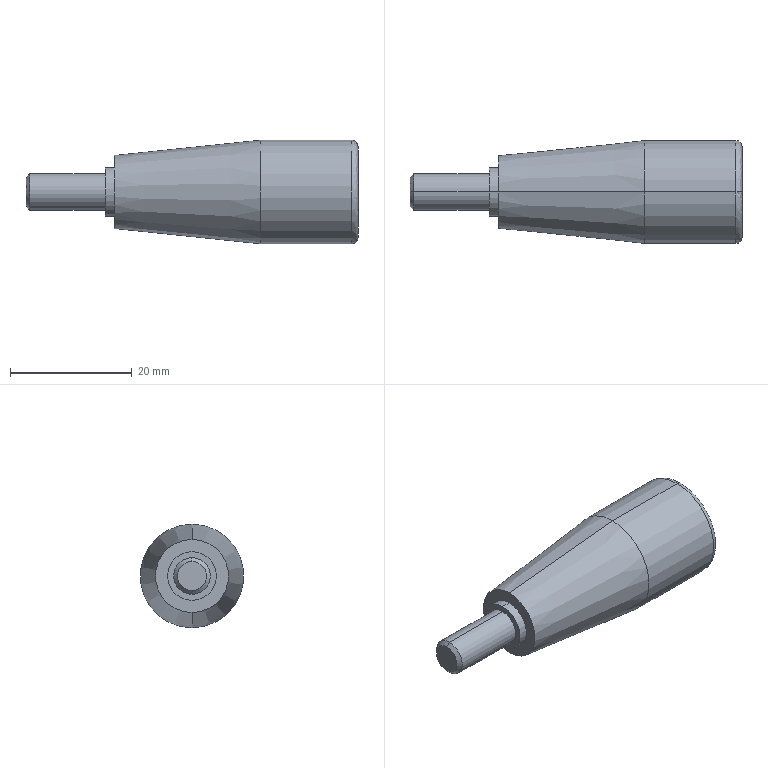Part | STEP file | GRAM6 | 1 solid | 20 faces | box 54.5 x 17 x 17 mm | volume 8003 mm3 | cylinder 8 | plane 6 | cone 4 | spline 2 | commonest cylinder face diameters 6 x2 6.5 x2 8 x2 17 x2
STEP:
#1=CARTESIAN_POINT('',(0.,0.,0.));
#2=DIRECTION('',(0.,0.,1.));
#3=DIRECTION('',(1.,0.,0.));
#4=AXIS2_PLACEMENT_3D('',#1,#2,#3);
#5=CARTESIAN_POINT('',(40.,0.,-7.5));
#6=VERTEX_POINT('',#5);
#7=CARTESIAN_POINT('',(40.,0.,7.5));
#8=VERTEX_POINT('',#7);
#9=CARTESIAN_POINT('',(40.,0.,-7.5));
#10=CARTESIAN_POINT('',(40.,-15.,-7.5));
#11=CARTESIAN_POINT('',(40.,-15.,7.5));
#12=CARTESIAN_POINT('',(40.,0.,7.5));
#13=(BOUNDED_CURVE()B_SPLINE_CURVE(3,(#9,#10,#11,#12),.UNSPECIFIED.,.F.,.F.)B_SPLINE_CURVE_WITH_KNOTS((4,4),(0.25,0.75),.PIECEWISE_BEZIER_KNOTS.)CURVE()GEOMETRIC_REPRESENTATION_ITEM()RATIONAL_B_SPLINE_CURVE((1.,0.3333,0.3333,1.))REPRESENTATION_ITEM(''));
#14=CARTESIAN_POINT('',(40.,0.,7.5));
#15=CARTESIAN_POINT('',(40.,-15.,7.5));
#16=CARTESIAN_POINT('',(40.,-15.,-7.5));
#17=CARTESIAN_POINT('',(40.,0.,-7.5));
#18=CARTESIAN_POINT('',(40.,0.,8.086));
#19=CARTESIAN_POINT('',(40.,-16.172,8.086));
#20=CARTESIAN_POINT('',(40.,-16.172,-8.086));
#21=CARTESIAN_POINT('',(40.,0.,-8.086));
#22=CARTESIAN_POINT('',(39.586,0.,8.5));
#23=CARTESIAN_POINT('',(39.586,-17.,8.5));
#24=CARTESIAN_POINT('',(39.586,-17.,-8.5));
#25=CARTESIAN_POINT('',(39.586,0.,-8.5));
#26=CARTESIAN_POINT('',(39.,0.,8.5));
#27=CARTESIAN_POINT('',(39.,-17.,8.5));
#28=CARTESIAN_POINT('',(39.,-17.,-8.5));
#29=CARTESIAN_POINT('',(39.,0.,-8.5));
#30=(BOUNDED_SURFACE()B_SPLINE_SURFACE(3,3,((#14,#15,#16,#17),(#18,#19,#20,#21),(#22,#23,#24,#25),(#26,#27,#28,#29)),.UNSPECIFIED.,.F.,.F.,.F.)B_SPLINE_SURFACE_WITH_KNOTS((4,4),(4,4),(0.,1.),(0.,1.),.PIECEWISE_BEZIER_KNOTS.)GEOMETRIC_REPRESENTATION_ITEM()RATIONAL_B_SPLINE_SURFACE(((1.,0.3333,0.3333,1.),(0.8047,0.2682,0.2682,0.8047),(0.8047,0.2682,0.2682,0.8047),(1.,0.3333,0.3333,1.)))REPRESENTATION_ITEM('')SURFACE());
#31=CARTESIAN_POINT('',(0.,1.));
#32=CARTESIAN_POINT('',(0.,0.));
#33=B_SPLINE_CURVE_WITH_KNOTS('',1,(#31,#32),.UNSPECIFIED.,.F.,.F.,(2,2),(0.25,0.75),.PIECEWISE_BEZIER_KNOTS.);
#34=(GEOMETRIC_REPRESENTATION_CONTEXT(2)PARAMETRIC_REPRESENTATION_CONTEXT()REPRESENTATION_CONTEXT('',''));
#35=DEFINITIONAL_REPRESENTATION('',(#33),#34);
#36=PCURVE('',#30,#35);
#37=CARTESIAN_POINT('',(40.,3.75,0.));
#38=DIRECTION('',(1.,0.,0.));
#39=DIRECTION('',(0.,0.,-1.));
#40=AXIS2_PLACEMENT_3D('',#37,#38,#39);
#41=PLANE('',#40);
#42=CARTESIAN_POINT('',(7.5,-3.75));
#43=CARTESIAN_POINT('',(7.5,-18.75));
#44=CARTESIAN_POINT('',(-7.5,-18.75));
#45=CARTESIAN_POINT('',(-7.5,-3.75));
#46=(BOUNDED_CURVE()B_SPLINE_CURVE(3,(#42,#43,#44,#45),.UNSPECIFIED.,.F.,.F.)B_SPLINE_CURVE_WITH_KNOTS((4,4),(0.25,0.75),.PIECEWISE_BEZIER_KNOTS.)CURVE()GEOMETRIC_REPRESENTATION_ITEM()RATIONAL_B_SPLINE_CURVE((1.,0.3333,0.3333,1.))REPRESENTATION_ITEM(''));
#47=(GEOMETRIC_REPRESENTATION_CONTEXT(2)PARAMETRIC_REPRESENTATION_CONTEXT()REPRESENTATION_CONTEXT('',''));
#48=DEFINITIONAL_REPRESENTATION('',(#46),#47);
#49=PCURVE('',#41,#48);
#50=SURFACE_CURVE('',#13,(#36,#49),.PCURVE_S1.);
#51=EDGE_CURVE('',#6,#8,#50,.T.);
#52=ORIENTED_EDGE('',*,*,#51,.T.);
#53=CARTESIAN_POINT('',(39.,0.,8.5));
#54=VERTEX_POINT('',#53);
#55=CARTESIAN_POINT('',(39.,0.,7.5));
#56=DIRECTION('',(0.,-1.,0.));
#57=DIRECTION('',(0.,0.,1.));
#58=AXIS2_PLACEMENT_3D('',#55,#56,#57);
#59=CIRCLE('',#58,1.);
#60=CARTESIAN_POINT('',(0.,0.));
#61=CARTESIAN_POINT('',(0.01683,0.));
#62=CARTESIAN_POINT('',(0.04999,0.));
#63=CARTESIAN_POINT('',(0.09843,0.));
#64=CARTESIAN_POINT('',(0.1457,0.));
#65=CARTESIAN_POINT('',(0.192,0.));
#66=CARTESIAN_POINT('',(0.2375,0.));
#67=CARTESIAN_POINT('',(0.2823,0.));
#68=CARTESIAN_POINT('',(0.3265,0.));
#69=CARTESIAN_POINT('',(0.3703,0.));
#70=CARTESIAN_POINT('',(0.4137,0.));
#71=CARTESIAN_POINT('',(0.4569,0.));
#72=CARTESIAN_POINT('',(0.5,0.));
#73=CARTESIAN_POINT('',(0.5431,0.));
#74=CARTESIAN_POINT('',(0.5863,0.));
#75=CARTESIAN_POINT('',(0.6297,0.));
#76=CARTESIAN_POINT('',(0.6735,0.));
#77=CARTESIAN_POINT('',(0.7177,0.));
#78=CARTESIAN_POINT('',(0.7625,0.));
#79=CARTESIAN_POINT('',(0.808,0.));
#80=CARTESIAN_POINT('',(0.8543,0.));
#81=CARTESIAN_POINT('',(0.9016,0.));
#82=CARTESIAN_POINT('',(0.95,0.));
#83=CARTESIAN_POINT('',(0.9832,0.));
#84=CARTESIAN_POINT('',(1.,0.));
#85=B_SPLINE_CURVE_WITH_KNOTS('',3,(#60,#61,#62,#63,#64,#65,#66,#67,#68,#69,#70,#71,#72,#73,#74,#75,#76,#77,#78,#79,#80,#81,#82,#83,#84),.UNSPECIFIED.,.F.,.F.,(4,1,1,1,1,1,1,1,1,1,1,1,1,1,1,1,1,1,1,1,1,1,4),(4.712,4.784,4.855,4.927,4.998,5.069,5.141,5.212,5.284,5.355,5.426,5.498,5.569,5.641,5.712,5.783,5.855,5.926,5.998,6.069,6.14,6.212,6.283),.QUASI_UNIFORM_KNOTS.);
#86=(GEOMETRIC_REPRESENTATION_CONTEXT(2)PARAMETRIC_REPRESENTATION_CONTEXT()REPRESENTATION_CONTEXT('',''));
#87=DEFINITIONAL_REPRESENTATION('',(#85),#86);
#88=PCURVE('',#30,#87);
#89=CARTESIAN_POINT('',(40.,0.,-7.5));
#90=CARTESIAN_POINT('',(40.,15.,-7.5));
#91=CARTESIAN_POINT('',(40.,15.,7.5));
#92=CARTESIAN_POINT('',(40.,0.,7.5));
#93=CARTESIAN_POINT('',(40.,0.,-8.086));
#94=CARTESIAN_POINT('',(40.,16.172,-8.086));
#95=CARTESIAN_POINT('',(40.,16.172,8.086));
#96=CARTESIAN_POINT('',(40.,0.,8.086));
#97=CARTESIAN_POINT('',(39.586,0.,-8.5));
#98=CARTESIAN_POINT('',(39.586,17.,-8.5));
#99=CARTESIAN_POINT('',(39.586,17.,8.5));
#100=CARTESIAN_POINT('',(39.586,0.,8.5));
#101=CARTESIAN_POINT('',(39.,0.,-8.5));
#102=CARTESIAN_POINT('',(39.,17.,-8.5));
#103=CARTESIAN_POINT('',(39.,17.,8.5));
#104=CARTESIAN_POINT('',(39.,0.,8.5));
#105=(BOUNDED_SURFACE()B_SPLINE_SURFACE(3,3,((#89,#90,#91,#92),(#93,#94,#95,#96),(#97,#98,#99,#100),(#101,#102,#103,#104)),.UNSPECIFIED.,.F.,.F.,.F.)B_SPLINE_SURFACE_WITH_KNOTS((4,4),(4,4),(0.,1.),(0.,1.),.PIECEWISE_BEZIER_KNOTS.)GEOMETRIC_REPRESENTATION_ITEM()RATIONAL_B_SPLINE_SURFACE(((1.,0.3333,0.3333,1.),(0.8047,0.2682,0.2682,0.8047),(0.8047,0.2682,0.2682,0.8047),(1.,0.3333,0.3333,1.)))REPRESENTATION_ITEM('')SURFACE());
#106=CARTESIAN_POINT('',(0.,1.));
#107=CARTESIAN_POINT('',(0.01683,1.));
#108=CARTESIAN_POINT('',(0.04999,1.));
#109=CARTESIAN_POINT('',(0.09843,1.));
#110=CARTESIAN_POINT('',(0.1457,1.));
#111=CARTESIAN_POINT('',(0.192,1.));
#112=CARTESIAN_POINT('',(0.2375,1.));
#113=CARTESIAN_POINT('',(0.2823,1.));
#114=CARTESIAN_POINT('',(0.3265,1.));
#115=CARTESIAN_POINT('',(0.3703,1.));
#116=CARTESIAN_POINT('',(0.4137,1.));
#117=CARTESIAN_POINT('',(0.4569,1.));
#118=CARTESIAN_POINT('',(0.5,1.));
#119=CARTESIAN_POINT('',(0.5431,1.));
#120=CARTESIAN_POINT('',(0.5863,1.));
#121=CARTESIAN_POINT('',(0.6297,1.));
#122=CARTESIAN_POINT('',(0.6735,1.));
#123=CARTESIAN_POINT('',(0.7177,1.));
#124=CARTESIAN_POINT('',(0.7625,1.));
#125=CARTESIAN_POINT('',(0.808,1.));
#126=CARTESIAN_POINT('',(0.8543,1.));
#127=CARTESIAN_POINT('',(0.9016,1.));
#128=CARTESIAN_POINT('',(0.95,1.));
#129=CARTESIAN_POINT('',(0.9832,1.));
#130=CARTESIAN_POINT('',(1.,1.));
#131=B_SPLINE_CURVE_WITH_KNOTS('',3,(#106,#107,#108,#109,#110,#111,#112,#113,#114,#115,#116,#117,#118,#119,#120,#121,#122,#123,#124,#125,#126,#127,#128,#129,#130),.UNSPECIFIED.,.F.,.F.,(4,1,1,1,1,1,1,1,1,1,1,1,1,1,1,1,1,1,1,1,1,1,4),(4.712,4.784,4.855,4.927,4.998,5.069,5.141,5.212,5.284,5.355,5.426,5.498,5.569,5.641,5.712,5.783,5.855,5.926,5.998,6.069,6.14,6.212,6.283),.QUASI_UNIFORM_KNOTS.);
#132=(GEOMETRIC_REPRESENTATION_CONTEXT(2)PARAMETRIC_REPRESENTATION_CONTEXT()REPRESENTATION_CONTEXT('',''));
#133=DEFINITIONAL_REPRESENTATION('',(#131),#132);
#134=PCURVE('',#105,#133);
#135=SURFACE_CURVE('',#59,(#88,#134),.PCURVE_S1.);
#136=EDGE_CURVE('',#8,#54,#135,.T.);
#137=ORIENTED_EDGE('',*,*,#136,.T.);
#138=CARTESIAN_POINT('',(39.,0.,-8.5));
#139=VERTEX_POINT('',#138);
#140=CARTESIAN_POINT('',(39.,0.,0.));
#141=DIRECTION('',(-1.,0.,0.));
#142=DIRECTION('',(0.,0.,-1.));
#143=AXIS2_PLACEMENT_3D('',#140,#141,#142);
#144=CIRCLE('',#143,8.5);
#145=CARTESIAN_POINT('',(1.,1.));
#146=CARTESIAN_POINT('',(1.,0.9763));
#147=CARTESIAN_POINT('',(1.,0.9319));
#148=CARTESIAN_POINT('',(1.,0.8733));
#149=CARTESIAN_POINT('',(1.,0.8206));
#150=CARTESIAN_POINT('',(1.,0.7724));
#151=CARTESIAN_POINT('',(1.,0.7279));
#152=CARTESIAN_POINT('',(1.,0.6861));
#153=CARTESIAN_POINT('',(1.,0.6465));
#154=CARTESIAN_POINT('',(1.,0.6086));
#155=CARTESIAN_POINT('',(1.,0.5718));
#156=CARTESIAN_POINT('',(1.,0.5357));
#157=CARTESIAN_POINT('',(1.,0.5));
#158=CARTESIAN_POINT('',(1.,0.4643));
#159=CARTESIAN_POINT('',(1.,0.4282));
#160=CARTESIAN_POINT('',(1.,0.3914));
#161=CARTESIAN_POINT('',(1.,0.3535));
#162=CARTESIAN_POINT('',(1.,0.3139));
#163=CARTESIAN_POINT('',(1.,0.2721));
#164=CARTESIAN_POINT('',(1.,0.2276));
#165=CARTESIAN_POINT('',(1.,0.1794));
#166=CARTESIAN_POINT('',(1.,0.1267));
#167=CARTESIAN_POINT('',(1.,0.06805));
#168=CARTESIAN_POINT('',(1.,0.02375));
#169=CARTESIAN_POINT('',(1.,0.));
#170=B_SPLINE_CURVE_WITH_KNOTS('',3,(#145,#146,#147,#148,#149,#150,#151,#152,#153,#154,#155,#156,#157,#158,#159,#160,#161,#162,#163,#164,#165,#166,#167,#168,#169),.UNSPECIFIED.,.F.,.F.,(4,1,1,1,1,1,1,1,1,1,1,1,1,1,1,1,1,1,1,1,1,1,4),(0.,0.1428,0.2856,0.4284,0.5712,0.714,0.8568,0.9996,1.142,1.285,1.428,1.571,1.714,1.856,1.999,2.142,2.285,2.428,2.57,2.713,2.856,2.999,3.142),.QUASI_UNIFORM_KNOTS.);
#171=(GEOMETRIC_REPRESENTATION_CONTEXT(2)PARAMETRIC_REPRESENTATION_CONTEXT()REPRESENTATION_CONTEXT('',''));
#172=DEFINITIONAL_REPRESENTATION('',(#170),#171);
#173=PCURVE('',#30,#172);
#174=CARTESIAN_POINT('',(31.5,0.,0.));
#175=DIRECTION('',(1.,0.,0.));
#176=DIRECTION('',(0.,0.,-1.));
#177=AXIS2_PLACEMENT_3D('',#174,#175,#176);
#178=CYLINDRICAL_SURFACE('',#177,8.5);
#179=CARTESIAN_POINT('',(6.283,7.5));
#180=DIRECTION('',(-1.,0.));
#181=VECTOR('',#180,1.);
#182=LINE('',#179,#181);
#183=(GEOMETRIC_REPRESENTATION_CONTEXT(2)PARAMETRIC_REPRESENTATION_CONTEXT()REPRESENTATION_CONTEXT('',''));
#184=DEFINITIONAL_REPRESENTATION('',(#182),#183);
#185=PCURVE('',#178,#184);
#186=SURFACE_CURVE('',#144,(#173,#185),.PCURVE_S1.);
#187=EDGE_CURVE('',#139,#54,#186,.T.);
#188=ORIENTED_EDGE('',*,*,#187,.F.);
#189=CARTESIAN_POINT('',(39.,0.,-7.5));
#190=DIRECTION('',(0.,1.,0.));
#191=DIRECTION('',(0.,0.,-1.));
#192=AXIS2_PLACEMENT_3D('',#189,#190,#191);
#193=CIRCLE('',#192,1.);
#194=CARTESIAN_POINT('',(0.,1.));
#195=CARTESIAN_POINT('',(0.01683,1.));
#196=CARTESIAN_POINT('',(0.04999,1.));
#197=CARTESIAN_POINT('',(0.09843,1.));
#198=CARTESIAN_POINT('',(0.1457,1.));
#199=CARTESIAN_POINT('',(0.192,1.));
#200=CARTESIAN_POINT('',(0.2375,1.));
#201=CARTESIAN_POINT('',(0.2823,1.));
#202=CARTESIAN_POINT('',(0.3265,1.));
#203=CARTESIAN_POINT('',(0.3703,1.));
#204=CARTESIAN_POINT('',(0.4137,1.));
#205=CARTESIAN_POINT('',(0.4569,1.));
#206=CARTESIAN_POINT('',(0.5,1.));
#207=CARTESIAN_POINT('',(0.5431,1.));
#208=CARTESIAN_POINT('',(0.5863,1.));
#209=CARTESIAN_POINT('',(0.6297,1.));
#210=CARTESIAN_POINT('',(0.6735,1.));
#211=CARTESIAN_POINT('',(0.7177,1.));
#212=CARTESIAN_POINT('',(0.7625,1.));
#213=CARTESIAN_POINT('',(0.808,1.));
#214=CARTESIAN_POINT('',(0.8543,1.));
#215=CARTESIAN_POINT('',(0.9016,1.));
#216=CARTESIAN_POINT('',(0.95,1.));
#217=CARTESIAN_POINT('',(0.9832,1.));
#218=CARTESIAN_POINT('',(1.,1.));
#219=B_SPLINE_CURVE_WITH_KNOTS('',3,(#194,#195,#196,#197,#198,#199,#200,#201,#202,#203,#204,#205,#206,#207,#208,#209,#210,#211,#212,#213,#214,#215,#216,#217,#218),.UNSPECIFIED.,.F.,.F.,(4,1,1,1,1,1,1,1,1,1,1,1,1,1,1,1,1,1,1,1,1,1,4),(4.712,4.784,4.855,4.927,4.998,5.069,5.141,5.212,5.284,5.355,5.426,5.498,5.569,5.641,5.712,5.783,5.855,5.926,5.998,6.069,6.14,6.212,6.283),.QUASI_UNIFORM_KNOTS.);
#220=(GEOMETRIC_REPRESENTATION_CONTEXT(2)PARAMETRIC_REPRESENTATION_CONTEXT()REPRESENTATION_CONTEXT('',''));
#221=DEFINITIONAL_REPRESENTATION('',(#219),#220);
#222=PCURVE('',#30,#221);
#223=CARTESIAN_POINT('',(0.,0.));
#224=CARTESIAN_POINT('',(0.01683,0.));
#225=CARTESIAN_POINT('',(0.04999,0.));
#226=CARTESIAN_POINT('',(0.09843,0.));
#227=CARTESIAN_POINT('',(0.1457,0.));
#228=CARTESIAN_POINT('',(0.192,0.));
#229=CARTESIAN_POINT('',(0.2375,0.));
#230=CARTESIAN_POINT('',(0.2823,0.));
#231=CARTESIAN_POINT('',(0.3265,0.));
#232=CARTESIAN_POINT('',(0.3703,0.));
#233=CARTESIAN_POINT('',(0.4137,0.));
#234=CARTESIAN_POINT('',(0.4569,0.));
#235=CARTESIAN_POINT('',(0.5,0.));
#236=CARTESIAN_POINT('',(0.5431,0.));
#237=CARTESIAN_POINT('',(0.5863,0.));
#238=CARTESIAN_POINT('',(0.6297,0.));
#239=CARTESIAN_POINT('',(0.6735,0.));
#240=CARTESIAN_POINT('',(0.7177,0.));
#241=CARTESIAN_POINT('',(0.7625,0.));
#242=CARTESIAN_POINT('',(0.808,0.));
#243=CARTESIAN_POINT('',(0.8543,0.));
#244=CARTESIAN_POINT('',(0.9016,0.));
#245=CARTESIAN_POINT('',(0.95,0.));
#246=CARTESIAN_POINT('',(0.9832,0.));
#247=CARTESIAN_POINT('',(1.,0.));
#248=B_SPLINE_CURVE_WITH_KNOTS('',3,(#223,#224,#225,#226,#227,#228,#229,#230,#231,#232,#233,#234,#235,#236,#237,#238,#239,#240,#241,#242,#243,#244,#245,#246,#247),.UNSPECIFIED.,.F.,.F.,(4,1,1,1,1,1,1,1,1,1,1,1,1,1,1,1,1,1,1,1,1,1,4),(4.712,4.784,4.855,4.927,4.998,5.069,5.141,5.212,5.284,5.355,5.426,5.498,5.569,5.641,5.712,5.783,5.855,5.926,5.998,6.069,6.14,6.212,6.283),.QUASI_UNIFORM_KNOTS.);
#249=(GEOMETRIC_REPRESENTATION_CONTEXT(2)PARAMETRIC_REPRESENTATION_CONTEXT()REPRESENTATION_CONTEXT('',''));
#250=DEFINITIONAL_REPRESENTATION('',(#248),#249);
#251=PCURVE('',#105,#250);
#252=SURFACE_CURVE('',#193,(#222,#251),.PCURVE_S1.);
#253=EDGE_CURVE('',#6,#139,#252,.T.);
#254=ORIENTED_EDGE('',*,*,#253,.F.);
#255=EDGE_LOOP('',(#52,#137,#188,#254));
#256=FACE_BOUND('',#255,.T.);
#257=ADVANCED_FACE('',(#256),#30,.T.);
#258=CARTESIAN_POINT('',(0.,0.,-6.));
#259=VERTEX_POINT('',#258);
#260=CARTESIAN_POINT('',(0.,0.,6.));
#261=VERTEX_POINT('',#260);
#262=CARTESIAN_POINT('',(0.,0.,0.));
#263=DIRECTION('',(1.,0.,0.));
#264=DIRECTION('',(0.,0.,-1.));
#265=AXIS2_PLACEMENT_3D('',#262,#263,#264);
#266=CIRCLE('',#265,6.);
#267=CARTESIAN_POINT('',(24.,0.,0.));
#268=DIRECTION('',(1.,0.,0.));
#269=DIRECTION('',(0.,0.,-1.));
#270=AXIS2_PLACEMENT_3D('',#267,#268,#269);
#271=CONICAL_SURFACE('',#270,8.5,0.1038);
#272=CARTESIAN_POINT('',(0.,-24.));
#273=DIRECTION('',(1.,0.));
#274=VECTOR('',#273,1.);
#275=LINE('',#272,#274);
#276=(GEOMETRIC_REPRESENTATION_CONTEXT(2)PARAMETRIC_REPRESENTATION_CONTEXT()REPRESENTATION_CONTEXT('',''));
#277=DEFINITIONAL_REPRESENTATION('',(#275),#276);
#278=PCURVE('',#271,#277);
#279=CARTESIAN_POINT('',(0.,3.,0.));
#280=DIRECTION('',(-1.,0.,0.));
#281=DIRECTION('',(0.,0.,1.));
#282=AXIS2_PLACEMENT_3D('',#279,#280,#281);
#283=PLANE('',#282);
#284=CARTESIAN_POINT('',(-6.,-3.));
#285=CARTESIAN_POINT('',(-6.,7.392));
#286=CARTESIAN_POINT('',(3.,2.196));
#287=CARTESIAN_POINT('',(12.,-3.));
#288=CARTESIAN_POINT('',(3.,-8.196));
#289=CARTESIAN_POINT('',(-6.,-13.392));
#290=CARTESIAN_POINT('',(-6.,-3.));
#291=(BOUNDED_CURVE()B_SPLINE_CURVE(2,(#284,#285,#286,#287,#288,#289,#290),.UNSPECIFIED.,.T.,.F.)B_SPLINE_CURVE_WITH_KNOTS((1,2,2,2,2,1),(-2.094,0.,2.094,4.189,6.283,8.378),.UNSPECIFIED.)CURVE()GEOMETRIC_REPRESENTATION_ITEM()RATIONAL_B_SPLINE_CURVE((1.,0.5,1.,0.5,1.,0.5,1.))REPRESENTATION_ITEM(''));
#292=(GEOMETRIC_REPRESENTATION_CONTEXT(2)PARAMETRIC_REPRESENTATION_CONTEXT()REPRESENTATION_CONTEXT('',''));
#293=DEFINITIONAL_REPRESENTATION('',(#291),#292);
#294=PCURVE('',#283,#293);
#295=SURFACE_CURVE('',#266,(#278,#294),.PCURVE_S1.);
#296=EDGE_CURVE('',#259,#261,#295,.T.);
#297=ORIENTED_EDGE('',*,*,#296,.T.);
#298=CARTESIAN_POINT('',(24.,0.,8.5));
#299=VERTEX_POINT('',#298);
#300=CARTESIAN_POINT('',(24.,0.,8.5));
#301=DIRECTION('',(0.9946,0.,0.1036));
#302=VECTOR('',#301,1.);
#303=LINE('',#300,#302);
#304=CARTESIAN_POINT('',(3.142,0.));
#305=DIRECTION('',(0.,1.));
#306=VECTOR('',#305,1.);
#307=LINE('',#304,#306);
#308=(GEOMETRIC_REPRESENTATION_CONTEXT(2)PARAMETRIC_REPRESENTATION_CONTEXT()REPRESENTATION_CONTEXT('',''));
#309=DEFINITIONAL_REPRESENTATION('',(#307),#308);
#310=PCURVE('',#271,#309);
#311=CARTESIAN_POINT('',(24.,0.,0.));
#312=DIRECTION('',(1.,0.,0.));
#313=DIRECTION('',(0.,0.,-1.));
#314=AXIS2_PLACEMENT_3D('',#311,#312,#313);
#315=CONICAL_SURFACE('',#314,8.5,0.1038);
#316=CARTESIAN_POINT('',(3.142,0.));
#317=DIRECTION('',(0.,1.));
#318=VECTOR('',#317,1.);
#319=LINE('',#316,#318);
#320=(GEOMETRIC_REPRESENTATION_CONTEXT(2)PARAMETRIC_REPRESENTATION_CONTEXT()REPRESENTATION_CONTEXT('',''));
#321=DEFINITIONAL_REPRESENTATION('',(#319),#320);
#322=PCURVE('',#315,#321);
#323=SURFACE_CURVE('',#303,(#310,#322),.PCURVE_S1.);
#324=EDGE_CURVE('',#261,#299,#323,.T.);
#325=ORIENTED_EDGE('',*,*,#324,.T.);
#326=CARTESIAN_POINT('',(24.,0.,-8.5));
#327=VERTEX_POINT('',#326);
#328=CARTESIAN_POINT('',(24.,0.,0.));
#329=DIRECTION('',(-1.,0.,0.));
#330=DIRECTION('',(0.,1.,0.));
#331=AXIS2_PLACEMENT_3D('',#328,#329,#330);
#332=CIRCLE('',#331,8.5);
#333=CARTESIAN_POINT('',(7.854,0.));
#334=DIRECTION('',(-1.,0.));
#335=VECTOR('',#334,1.);
#336=LINE('',#333,#335);
#337=(GEOMETRIC_REPRESENTATION_CONTEXT(2)PARAMETRIC_REPRESENTATION_CONTEXT()REPRESENTATION_CONTEXT('',''));
#338=DEFINITIONAL_REPRESENTATION('',(#336),#337);
#339=PCURVE('',#271,#338);
#340=CARTESIAN_POINT('',(31.5,0.,0.));
#341=DIRECTION('',(1.,0.,0.));
#342=DIRECTION('',(0.,0.,-1.));
#343=AXIS2_PLACEMENT_3D('',#340,#341,#342);
#344=CYLINDRICAL_SURFACE('',#343,8.5);
#345=CARTESIAN_POINT('',(7.854,-7.5));
#346=DIRECTION('',(-1.,0.));
#347=VECTOR('',#346,1.);
#348=LINE('',#345,#347);
#349=(GEOMETRIC_REPRESENTATION_CONTEXT(2)PARAMETRIC_REPRESENTATION_CONTEXT()REPRESENTATION_CONTEXT('',''));
#350=DEFINITIONAL_REPRESENTATION('',(#348),#349);
#351=PCURVE('',#344,#350);
#352=SURFACE_CURVE('',#332,(#339,#351),.PCURVE_S1.);
#353=EDGE_CURVE('',#299,#327,#352,.T.);
#354=ORIENTED_EDGE('',*,*,#353,.T.);
#355=CARTESIAN_POINT('',(24.,0.,-8.5));
#356=DIRECTION('',(0.9946,0.,-0.1036));
#357=VECTOR('',#356,1.);
#358=LINE('',#355,#357);
#359=CARTESIAN_POINT('',(0.,0.));
#360=DIRECTION('',(0.,1.));
#361=VECTOR('',#360,1.);
#362=LINE('',#359,#361);
#363=(GEOMETRIC_REPRESENTATION_CONTEXT(2)PARAMETRIC_REPRESENTATION_CONTEXT()REPRESENTATION_CONTEXT('',''));
#364=DEFINITIONAL_REPRESENTATION('',(#362),#363);
#365=PCURVE('',#271,#364);
#366=CARTESIAN_POINT('',(6.283,0.));
#367=DIRECTION('',(0.,1.));
#368=VECTOR('',#367,1.);
#369=LINE('',#366,#368);
#370=(GEOMETRIC_REPRESENTATION_CONTEXT(2)PARAMETRIC_REPRESENTATION_CONTEXT()REPRESENTATION_CONTEXT('',''));
#371=DEFINITIONAL_REPRESENTATION('',(#369),#370);
#372=PCURVE('',#315,#371);
#373=SURFACE_CURVE('',#358,(#365,#372),.PCURVE_S1.);
#374=EDGE_CURVE('',#259,#327,#373,.T.);
#375=ORIENTED_EDGE('',*,*,#374,.F.);
#376=EDGE_LOOP('',(#297,#325,#354,#375));
#377=FACE_BOUND('',#376,.T.);
#378=ADVANCED_FACE('',(#377),#271,.T.);
#379=ORIENTED_EDGE('',*,*,#353,.F.);
#380=CARTESIAN_POINT('',(31.5,0.,8.5));
#381=DIRECTION('',(1.,0.,0.));
#382=VECTOR('',#381,1.);
#383=LINE('',#380,#382);
#384=CARTESIAN_POINT('',(3.142,0.));
#385=DIRECTION('',(0.,1.));
#386=VECTOR('',#385,1.);
#387=LINE('',#384,#386);
#388=(GEOMETRIC_REPRESENTATION_CONTEXT(2)PARAMETRIC_REPRESENTATION_CONTEXT()REPRESENTATION_CONTEXT('',''));
#389=DEFINITIONAL_REPRESENTATION('',(#387),#388);
#390=PCURVE('',#344,#389);
#391=CARTESIAN_POINT('',(3.142,0.));
#392=DIRECTION('',(0.,1.));
#393=VECTOR('',#392,1.);
#394=LINE('',#391,#393);
#395=(GEOMETRIC_REPRESENTATION_CONTEXT(2)PARAMETRIC_REPRESENTATION_CONTEXT()REPRESENTATION_CONTEXT('',''));
#396=DEFINITIONAL_REPRESENTATION('',(#394),#395);
#397=PCURVE('',#178,#396);
#398=SURFACE_CURVE('',#383,(#390,#397),.PCURVE_S1.);
#399=EDGE_CURVE('',#299,#54,#398,.T.);
#400=ORIENTED_EDGE('',*,*,#399,.T.);
#401=CARTESIAN_POINT('',(39.,0.,0.));
#402=DIRECTION('',(-1.,0.,0.));
#403=DIRECTION('',(0.,0.,-1.));
#404=AXIS2_PLACEMENT_3D('',#401,#402,#403);
#405=CIRCLE('',#404,8.5);
#406=CARTESIAN_POINT('',(6.283,7.5));
#407=DIRECTION('',(-1.,0.));
#408=VECTOR('',#407,1.);
#409=LINE('',#406,#408);
#410=(GEOMETRIC_REPRESENTATION_CONTEXT(2)PARAMETRIC_REPRESENTATION_CONTEXT()REPRESENTATION_CONTEXT('',''));
#411=DEFINITIONAL_REPRESENTATION('',(#409),#410);
#412=PCURVE('',#344,#411);
#413=CARTESIAN_POINT('',(1.,1.));
#414=CARTESIAN_POINT('',(1.,0.9763));
#415=CARTESIAN_POINT('',(1.,0.9319));
#416=CARTESIAN_POINT('',(1.,0.8733));
#417=CARTESIAN_POINT('',(1.,0.8206));
#418=CARTESIAN_POINT('',(1.,0.7724));
#419=CARTESIAN_POINT('',(1.,0.7279));
#420=CARTESIAN_POINT('',(1.,0.6861));
#421=CARTESIAN_POINT('',(1.,0.6465));
#422=CARTESIAN_POINT('',(1.,0.6086));
#423=CARTESIAN_POINT('',(1.,0.5718));
#424=CARTESIAN_POINT('',(1.,0.5357));
#425=CARTESIAN_POINT('',(1.,0.5));
#426=CARTESIAN_POINT('',(1.,0.4643));
#427=CARTESIAN_POINT('',(1.,0.4282));
#428=CARTESIAN_POINT('',(1.,0.3914));
#429=CARTESIAN_POINT('',(1.,0.3535));
#430=CARTESIAN_POINT('',(1.,0.3139));
#431=CARTESIAN_POINT('',(1.,0.2721));
#432=CARTESIAN_POINT('',(1.,0.2276));
#433=CARTESIAN_POINT('',(1.,0.1794));
#434=CARTESIAN_POINT('',(1.,0.1267));
#435=CARTESIAN_POINT('',(1.,0.06805));
#436=CARTESIAN_POINT('',(1.,0.02375));
#437=CARTESIAN_POINT('',(1.,0.));
#438=B_SPLINE_CURVE_WITH_KNOTS('',3,(#413,#414,#415,#416,#417,#418,#419,#420,#421,#422,#423,#424,#425,#426,#427,#428,#429,#430,#431,#432,#433,#434,#435,#436,#437),.UNSPECIFIED.,.F.,.F.,(4,1,1,1,1,1,1,1,1,1,1,1,1,1,1,1,1,1,1,1,1,1,4),(3.142,3.284,3.427,3.57,3.713,3.856,3.998,4.141,4.284,4.427,4.57,4.712,4.855,4.998,5.141,5.284,5.426,5.569,5.712,5.855,5.998,6.14,6.283),.QUASI_UNIFORM_KNOTS.);
#439=(GEOMETRIC_REPRESENTATION_CONTEXT(2)PARAMETRIC_REPRESENTATION_CONTEXT()REPRESENTATION_CONTEXT('',''));
#440=DEFINITIONAL_REPRESENTATION('',(#438),#439);
#441=PCURVE('',#105,#440);
#442=SURFACE_CURVE('',#405,(#412,#441),.PCURVE_S1.);
#443=EDGE_CURVE('',#54,#139,#442,.T.);
#444=ORIENTED_EDGE('',*,*,#443,.T.);
#445=CARTESIAN_POINT('',(31.5,0.,-8.5));
#446=DIRECTION('',(1.,0.,0.));
#447=VECTOR('',#446,1.);
#448=LINE('',#445,#447);
#449=CARTESIAN_POINT('',(0.,0.));
#450=DIRECTION('',(0.,1.));
#451=VECTOR('',#450,1.);
#452=LINE('',#449,#451);
#453=(GEOMETRIC_REPRESENTATION_CONTEXT(2)PARAMETRIC_REPRESENTATION_CONTEXT()REPRESENTATION_CONTEXT('',''));
#454=DEFINITIONAL_REPRESENTATION('',(#452),#453);
#455=PCURVE('',#344,#454);
#456=CARTESIAN_POINT('',(6.283,0.));
#457=DIRECTION('',(0.,1.));
#458=VECTOR('',#457,1.);
#459=LINE('',#456,#458);
#460=(GEOMETRIC_REPRESENTATION_CONTEXT(2)PARAMETRIC_REPRESENTATION_CONTEXT()REPRESENTATION_CONTEXT('',''));
#461=DEFINITIONAL_REPRESENTATION('',(#459),#460);
#462=PCURVE('',#178,#461);
#463=SURFACE_CURVE('',#448,(#455,#462),.PCURVE_S1.);
#464=EDGE_CURVE('',#327,#139,#463,.T.);
#465=ORIENTED_EDGE('',*,*,#464,.F.);
#466=EDGE_LOOP('',(#379,#400,#444,#465));
#467=FACE_BOUND('',#466,.T.);
#468=ADVANCED_FACE('',(#467),#344,.T.);
#469=CARTESIAN_POINT('',(-1.5,0.,-4.));
#470=VERTEX_POINT('',#469);
#471=CARTESIAN_POINT('',(-1.5,0.,4.));
#472=VERTEX_POINT('',#471);
#473=CARTESIAN_POINT('',(-1.5,0.,0.));
#474=DIRECTION('',(1.,0.,0.));
#475=DIRECTION('',(0.,0.,-1.));
#476=AXIS2_PLACEMENT_3D('',#473,#474,#475);
#477=CIRCLE('',#476,4.);
#478=CARTESIAN_POINT('',(0.,0.,0.));
#479=DIRECTION('',(1.,0.,0.));
#480=DIRECTION('',(0.,0.,-1.));
#481=AXIS2_PLACEMENT_3D('',#478,#479,#480);
#482=CYLINDRICAL_SURFACE('',#481,4.);
#483=CARTESIAN_POINT('',(0.,-1.5));
#484=DIRECTION('',(1.,0.));
#485=VECTOR('',#484,1.);
#486=LINE('',#483,#485);
#487=(GEOMETRIC_REPRESENTATION_CONTEXT(2)PARAMETRIC_REPRESENTATION_CONTEXT()REPRESENTATION_CONTEXT('',''));
#488=DEFINITIONAL_REPRESENTATION('',(#486),#487);
#489=PCURVE('',#482,#488);
#490=CARTESIAN_POINT('',(-1.5,3.5,0.));
#491=DIRECTION('',(-1.,0.,0.));
#492=DIRECTION('',(0.,0.,1.));
#493=AXIS2_PLACEMENT_3D('',#490,#491,#492);
#494=PLANE('',#493);
#495=CARTESIAN_POINT('',(-4.,-3.5));
#496=CARTESIAN_POINT('',(-4.,3.428));
#497=CARTESIAN_POINT('',(2.,-0.0359));
#498=CARTESIAN_POINT('',(8.,-3.5));
#499=CARTESIAN_POINT('',(2.,-6.964));
#500=CARTESIAN_POINT('',(-4.,-10.428));
#501=CARTESIAN_POINT('',(-4.,-3.5));
#502=(BOUNDED_CURVE()B_SPLINE_CURVE(2,(#495,#496,#497,#498,#499,#500,#501),.UNSPECIFIED.,.T.,.F.)B_SPLINE_CURVE_WITH_KNOTS((1,2,2,2,2,1),(-2.094,0.,2.094,4.189,6.283,8.378),.UNSPECIFIED.)CURVE()GEOMETRIC_REPRESENTATION_ITEM()RATIONAL_B_SPLINE_CURVE((1.,0.5,1.,0.5,1.,0.5,1.))REPRESENTATION_ITEM(''));
#503=(GEOMETRIC_REPRESENTATION_CONTEXT(2)PARAMETRIC_REPRESENTATION_CONTEXT()REPRESENTATION_CONTEXT('',''));
#504=DEFINITIONAL_REPRESENTATION('',(#502),#503);
#505=PCURVE('',#494,#504);
#506=SURFACE_CURVE('',#477,(#489,#505),.PCURVE_S1.);
#507=EDGE_CURVE('',#470,#472,#506,.T.);
#508=ORIENTED_EDGE('',*,*,#507,.T.);
#509=CARTESIAN_POINT('',(0.,0.,4.));
#510=VERTEX_POINT('',#509);
#511=CARTESIAN_POINT('',(0.,0.,4.));
#512=DIRECTION('',(1.,0.,0.));
#513=VECTOR('',#512,1.);
#514=LINE('',#511,#513);
#515=CARTESIAN_POINT('',(3.142,0.));
#516=DIRECTION('',(0.,1.));
#517=VECTOR('',#516,1.);
#518=LINE('',#515,#517);
#519=(GEOMETRIC_REPRESENTATION_CONTEXT(2)PARAMETRIC_REPRESENTATION_CONTEXT()REPRESENTATION_CONTEXT('',''));
#520=DEFINITIONAL_REPRESENTATION('',(#518),#519);
#521=PCURVE('',#482,#520);
#522=CARTESIAN_POINT('',(0.,0.,0.));
#523=DIRECTION('',(1.,0.,0.));
#524=DIRECTION('',(0.,0.,-1.));
#525=AXIS2_PLACEMENT_3D('',#522,#523,#524);
#526=CYLINDRICAL_SURFACE('',#525,4.);
#527=CARTESIAN_POINT('',(3.142,0.));
#528=DIRECTION('',(0.,1.));
#529=VECTOR('',#528,1.);
#530=LINE('',#527,#529);
#531=(GEOMETRIC_REPRESENTATION_CONTEXT(2)PARAMETRIC_REPRESENTATION_CONTEXT()REPRESENTATION_CONTEXT('',''));
#532=DEFINITIONAL_REPRESENTATION('',(#530),#531);
#533=PCURVE('',#526,#532);
#534=SURFACE_CURVE('',#514,(#521,#533),.PCURVE_S1.);
#535=EDGE_CURVE('',#472,#510,#534,.T.);
#536=ORIENTED_EDGE('',*,*,#535,.T.);
#537=CARTESIAN_POINT('',(0.,0.,-4.));
#538=VERTEX_POINT('',#537);
#539=CARTESIAN_POINT('',(0.,0.,0.));
#540=DIRECTION('',(1.,0.,0.));
#541=DIRECTION('',(0.,0.,-1.));
#542=AXIS2_PLACEMENT_3D('',#539,#540,#541);
#543=CIRCLE('',#542,4.);
#544=CARTESIAN_POINT('',(0.,0.));
#545=DIRECTION('',(1.,0.));
#546=VECTOR('',#545,1.);
#547=LINE('',#544,#546);
#548=(GEOMETRIC_REPRESENTATION_CONTEXT(2)PARAMETRIC_REPRESENTATION_CONTEXT()REPRESENTATION_CONTEXT('',''));
#549=DEFINITIONAL_REPRESENTATION('',(#547),#548);
#550=PCURVE('',#482,#549);
#551=CARTESIAN_POINT('',(-4.,-3.));
#552=CARTESIAN_POINT('',(-4.,3.928));
#553=CARTESIAN_POINT('',(2.,0.4641));
#554=CARTESIAN_POINT('',(8.,-3.));
#555=CARTESIAN_POINT('',(2.,-6.464));
#556=CARTESIAN_POINT('',(-4.,-9.928));
#557=CARTESIAN_POINT('',(-4.,-3.));
#558=(BOUNDED_CURVE()B_SPLINE_CURVE(2,(#551,#552,#553,#554,#555,#556,#557),.UNSPECIFIED.,.T.,.F.)B_SPLINE_CURVE_WITH_KNOTS((1,2,2,2,2,1),(-2.094,0.,2.094,4.189,6.283,8.378),.UNSPECIFIED.)CURVE()GEOMETRIC_REPRESENTATION_ITEM()RATIONAL_B_SPLINE_CURVE((1.,0.5,1.,0.5,1.,0.5,1.))REPRESENTATION_ITEM(''));
#559=(GEOMETRIC_REPRESENTATION_CONTEXT(2)PARAMETRIC_REPRESENTATION_CONTEXT()REPRESENTATION_CONTEXT('',''));
#560=DEFINITIONAL_REPRESENTATION('',(#558),#559);
#561=PCURVE('',#283,#560);
#562=SURFACE_CURVE('',#543,(#550,#561),.PCURVE_S1.);
#563=EDGE_CURVE('',#538,#510,#562,.T.);
#564=ORIENTED_EDGE('',*,*,#563,.F.);
#565=CARTESIAN_POINT('',(0.,0.,-4.));
#566=DIRECTION('',(1.,0.,0.));
#567=VECTOR('',#566,1.);
#568=LINE('',#565,#567);
#569=CARTESIAN_POINT('',(0.,0.));
#570=DIRECTION('',(0.,1.));
#571=VECTOR('',#570,1.);
#572=LINE('',#569,#571);
#573=(GEOMETRIC_REPRESENTATION_CONTEXT(2)PARAMETRIC_REPRESENTATION_CONTEXT()REPRESENTATION_CONTEXT('',''));
#574=DEFINITIONAL_REPRESENTATION('',(#572),#573);
#575=PCURVE('',#482,#574);
#576=CARTESIAN_POINT('',(6.283,0.));
#577=DIRECTION('',(0.,1.));
#578=VECTOR('',#577,1.);
#579=LINE('',#576,#578);
#580=(GEOMETRIC_REPRESENTATION_CONTEXT(2)PARAMETRIC_REPRESENTATION_CONTEXT()REPRESENTATION_CONTEXT('',''));
#581=DEFINITIONAL_REPRESENTATION('',(#579),#580);
#582=PCURVE('',#526,#581);
#583=SURFACE_CURVE('',#568,(#575,#582),.PCURVE_S1.);
#584=EDGE_CURVE('',#470,#538,#583,.T.);
#585=ORIENTED_EDGE('',*,*,#584,.F.);
#586=EDGE_LOOP('',(#508,#536,#564,#585));
#587=FACE_BOUND('',#586,.T.);
#588=ADVANCED_FACE('',(#587),#482,.T.);
#589=CARTESIAN_POINT('',(-13.886,0.,-3.));
#590=VERTEX_POINT('',#589);
#591=CARTESIAN_POINT('',(-13.886,0.,3.));
#592=VERTEX_POINT('',#591);
#593=CARTESIAN_POINT('',(-13.886,0.,0.));
#594=DIRECTION('',(1.,0.,0.));
#595=DIRECTION('',(0.,0.,-1.));
#596=AXIS2_PLACEMENT_3D('',#593,#594,#595);
#597=CIRCLE('',#596,3.);
#598=CARTESIAN_POINT('',(-7.693,0.,0.));
#599=DIRECTION('',(1.,0.,0.));
#600=DIRECTION('',(0.,0.,-1.));
#601=AXIS2_PLACEMENT_3D('',#598,#599,#600);
#602=CYLINDRICAL_SURFACE('',#601,3.);
#603=CARTESIAN_POINT('',(0.,-6.193));
#604=DIRECTION('',(1.,0.));
#605=VECTOR('',#604,1.);
#606=LINE('',#603,#605);
#607=(GEOMETRIC_REPRESENTATION_CONTEXT(2)PARAMETRIC_REPRESENTATION_CONTEXT()REPRESENTATION_CONTEXT('',''));
#608=DEFINITIONAL_REPRESENTATION('',(#606),#607);
#609=PCURVE('',#602,#608);
#610=CARTESIAN_POINT('',(-13.886,0.,0.));
#611=DIRECTION('',(1.,0.,0.));
#612=DIRECTION('',(0.,0.,-1.));
#613=AXIS2_PLACEMENT_3D('',#610,#611,#612);
#614=CONICAL_SURFACE('',#613,3.,0.7854);
#615=CARTESIAN_POINT('',(0.,0.));
#616=DIRECTION('',(1.,0.));
#617=VECTOR('',#616,1.);
#618=LINE('',#615,#617);
#619=(GEOMETRIC_REPRESENTATION_CONTEXT(2)PARAMETRIC_REPRESENTATION_CONTEXT()REPRESENTATION_CONTEXT('',''));
#620=DEFINITIONAL_REPRESENTATION('',(#618),#619);
#621=PCURVE('',#614,#620);
#622=SURFACE_CURVE('',#597,(#609,#621),.PCURVE_S1.);
#623=EDGE_CURVE('',#590,#592,#622,.T.);
#624=ORIENTED_EDGE('',*,*,#623,.T.);
#625=CARTESIAN_POINT('',(-1.5,0.,3.));
#626=VERTEX_POINT('',#625);
#627=CARTESIAN_POINT('',(-7.693,0.,3.));
#628=DIRECTION('',(1.,0.,0.));
#629=VECTOR('',#628,1.);
#630=LINE('',#627,#629);
#631=CARTESIAN_POINT('',(3.142,0.));
#632=DIRECTION('',(0.,1.));
#633=VECTOR('',#632,1.);
#634=LINE('',#631,#633);
#635=(GEOMETRIC_REPRESENTATION_CONTEXT(2)PARAMETRIC_REPRESENTATION_CONTEXT()REPRESENTATION_CONTEXT('',''));
#636=DEFINITIONAL_REPRESENTATION('',(#634),#635);
#637=PCURVE('',#602,#636);
#638=CARTESIAN_POINT('',(-7.693,0.,0.));
#639=DIRECTION('',(1.,0.,0.));
#640=DIRECTION('',(0.,0.,-1.));
#641=AXIS2_PLACEMENT_3D('',#638,#639,#640);
#642=CYLINDRICAL_SURFACE('',#641,3.);
#643=CARTESIAN_POINT('',(3.142,0.));
#644=DIRECTION('',(0.,1.));
#645=VECTOR('',#644,1.);
#646=LINE('',#643,#645);
#647=(GEOMETRIC_REPRESENTATION_CONTEXT(2)PARAMETRIC_REPRESENTATION_CONTEXT()REPRESENTATION_CONTEXT('',''));
#648=DEFINITIONAL_REPRESENTATION('',(#646),#647);
#649=PCURVE('',#642,#648);
#650=SURFACE_CURVE('',#630,(#637,#649),.PCURVE_S1.);
#651=EDGE_CURVE('',#592,#626,#650,.T.);
#652=ORIENTED_EDGE('',*,*,#651,.T.);
#653=CARTESIAN_POINT('',(-1.5,0.,-3.));
#654=VERTEX_POINT('',#653);
#655=CARTESIAN_POINT('',(-1.5,0.,0.));
#656=DIRECTION('',(1.,0.,0.));
#657=DIRECTION('',(0.,0.,-1.));
#658=AXIS2_PLACEMENT_3D('',#655,#656,#657);
#659=CIRCLE('',#658,3.);
#660=CARTESIAN_POINT('',(0.,6.193));
#661=DIRECTION('',(1.,0.));
#662=VECTOR('',#661,1.);
#663=LINE('',#660,#662);
#664=(GEOMETRIC_REPRESENTATION_CONTEXT(2)PARAMETRIC_REPRESENTATION_CONTEXT()REPRESENTATION_CONTEXT('',''));
#665=DEFINITIONAL_REPRESENTATION('',(#663),#664);
#666=PCURVE('',#602,#665);
#667=CARTESIAN_POINT('',(-3.,-3.5));
#668=CARTESIAN_POINT('',(-3.,1.696));
#669=CARTESIAN_POINT('',(1.5,-0.9019));
#670=CARTESIAN_POINT('',(6.,-3.5));
#671=CARTESIAN_POINT('',(1.5,-6.098));
#672=CARTESIAN_POINT('',(-3.,-8.696));
#673=CARTESIAN_POINT('',(-3.,-3.5));
#674=(BOUNDED_CURVE()B_SPLINE_CURVE(2,(#667,#668,#669,#670,#671,#672,#673),.UNSPECIFIED.,.T.,.F.)B_SPLINE_CURVE_WITH_KNOTS((1,2,2,2,2,1),(-2.094,0.,2.094,4.189,6.283,8.378),.UNSPECIFIED.)CURVE()GEOMETRIC_REPRESENTATION_ITEM()RATIONAL_B_SPLINE_CURVE((1.,0.5,1.,0.5,1.,0.5,1.))REPRESENTATION_ITEM(''));
#675=(GEOMETRIC_REPRESENTATION_CONTEXT(2)PARAMETRIC_REPRESENTATION_CONTEXT()REPRESENTATION_CONTEXT('',''));
#676=DEFINITIONAL_REPRESENTATION('',(#674),#675);
#677=PCURVE('',#494,#676);
#678=SURFACE_CURVE('',#659,(#666,#677),.PCURVE_S1.);
#679=EDGE_CURVE('',#654,#626,#678,.T.);
#680=ORIENTED_EDGE('',*,*,#679,.F.);
#681=CARTESIAN_POINT('',(-7.693,0.,-3.));
#682=DIRECTION('',(1.,0.,0.));
#683=VECTOR('',#682,1.);
#684=LINE('',#681,#683);
#685=CARTESIAN_POINT('',(0.,0.));
#686=DIRECTION('',(0.,1.));
#687=VECTOR('',#686,1.);
#688=LINE('',#685,#687);
#689=(GEOMETRIC_REPRESENTATION_CONTEXT(2)PARAMETRIC_REPRESENTATION_CONTEXT()REPRESENTATION_CONTEXT('',''));
#690=DEFINITIONAL_REPRESENTATION('',(#688),#689);
#691=PCURVE('',#602,#690);
#692=CARTESIAN_POINT('',(6.283,0.));
#693=DIRECTION('',(0.,1.));
#694=VECTOR('',#693,1.);
#695=LINE('',#692,#694);
#696=(GEOMETRIC_REPRESENTATION_CONTEXT(2)PARAMETRIC_REPRESENTATION_CONTEXT()REPRESENTATION_CONTEXT('',''));
#697=DEFINITIONAL_REPRESENTATION('',(#695),#696);
#698=PCURVE('',#642,#697);
#699=SURFACE_CURVE('',#684,(#691,#698),.PCURVE_S1.);
#700=EDGE_CURVE('',#590,#654,#699,.T.);
#701=ORIENTED_EDGE('',*,*,#700,.F.);
#702=EDGE_LOOP('',(#624,#652,#680,#701));
#703=FACE_BOUND('',#702,.T.);
#704=ADVANCED_FACE('',(#703),#602,.T.);
#705=CARTESIAN_POINT('',(-14.5,0.,-2.387));
#706=VERTEX_POINT('',#705);
#707=CARTESIAN_POINT('',(-14.5,0.,2.387));
#708=VERTEX_POINT('',#707);
#709=CARTESIAN_POINT('',(-14.5,0.,0.));
#710=DIRECTION('',(1.,0.,0.));
#711=DIRECTION('',(0.,0.,-1.));
#712=AXIS2_PLACEMENT_3D('',#709,#710,#711);
#713=CIRCLE('',#712,2.387);
#714=CARTESIAN_POINT('',(0.,-0.6135));
#715=DIRECTION('',(1.,0.));
#716=VECTOR('',#715,1.);
#717=LINE('',#714,#716);
#718=(GEOMETRIC_REPRESENTATION_CONTEXT(2)PARAMETRIC_REPRESENTATION_CONTEXT()REPRESENTATION_CONTEXT('',''));
#719=DEFINITIONAL_REPRESENTATION('',(#717),#718);
#720=PCURVE('',#614,#719);
#721=CARTESIAN_POINT('',(-14.5,1.193,0.));
#722=DIRECTION('',(-1.,0.,0.));
#723=DIRECTION('',(0.,0.,1.));
#724=AXIS2_PLACEMENT_3D('',#721,#722,#723);
#725=PLANE('',#724);
#726=CARTESIAN_POINT('',(-2.387,-1.193));
#727=CARTESIAN_POINT('',(-2.387,2.94));
#728=CARTESIAN_POINT('',(1.193,0.8735));
#729=CARTESIAN_POINT('',(4.773,-1.193));
#730=CARTESIAN_POINT('',(1.193,-3.26));
#731=CARTESIAN_POINT('',(-2.387,-5.327));
#732=CARTESIAN_POINT('',(-2.387,-1.193));
#733=(BOUNDED_CURVE()B_SPLINE_CURVE(2,(#726,#727,#728,#729,#730,#731,#732),.UNSPECIFIED.,.T.,.F.)B_SPLINE_CURVE_WITH_KNOTS((1,2,2,2,2,1),(-2.094,0.,2.094,4.189,6.283,8.378),.UNSPECIFIED.)CURVE()GEOMETRIC_REPRESENTATION_ITEM()RATIONAL_B_SPLINE_CURVE((1.,0.5,1.,0.5,1.,0.5,1.))REPRESENTATION_ITEM(''));
#734=(GEOMETRIC_REPRESENTATION_CONTEXT(2)PARAMETRIC_REPRESENTATION_CONTEXT()REPRESENTATION_CONTEXT('',''));
#735=DEFINITIONAL_REPRESENTATION('',(#733),#734);
#736=PCURVE('',#725,#735);
#737=SURFACE_CURVE('',#713,(#720,#736),.PCURVE_S1.);
#738=EDGE_CURVE('',#706,#708,#737,.T.);
#739=ORIENTED_EDGE('',*,*,#738,.T.);
#740=CARTESIAN_POINT('',(-13.886,0.,3.));
#741=DIRECTION('',(0.7071,0.,0.7071));
#742=VECTOR('',#741,1.);
#743=LINE('',#740,#742);
#744=CARTESIAN_POINT('',(3.142,0.));
#745=DIRECTION('',(0.,1.));
#746=VECTOR('',#745,1.);
#747=LINE('',#744,#746);
#748=(GEOMETRIC_REPRESENTATION_CONTEXT(2)PARAMETRIC_REPRESENTATION_CONTEXT()REPRESENTATION_CONTEXT('',''));
#749=DEFINITIONAL_REPRESENTATION('',(#747),#748);
#750=PCURVE('',#614,#749);
#751=CARTESIAN_POINT('',(-13.886,0.,0.));
#752=DIRECTION('',(1.,0.,0.));
#753=DIRECTION('',(0.,0.,-1.));
#754=AXIS2_PLACEMENT_3D('',#751,#752,#753);
#755=CONICAL_SURFACE('',#754,3.,0.7854);
#756=CARTESIAN_POINT('',(3.142,0.));
#757=DIRECTION('',(0.,1.));
#758=VECTOR('',#757,1.);
#759=LINE('',#756,#758);
#760=(GEOMETRIC_REPRESENTATION_CONTEXT(2)PARAMETRIC_REPRESENTATION_CONTEXT()REPRESENTATION_CONTEXT('',''));
#761=DEFINITIONAL_REPRESENTATION('',(#759),#760);
#762=PCURVE('',#755,#761);
#763=SURFACE_CURVE('',#743,(#750,#762),.PCURVE_S1.);
#764=EDGE_CURVE('',#708,#592,#763,.T.);
#765=ORIENTED_EDGE('',*,*,#764,.T.);
#766=ORIENTED_EDGE('',*,*,#623,.F.);
#767=CARTESIAN_POINT('',(-13.886,0.,-3.));
#768=DIRECTION('',(0.7071,0.,-0.7071));
#769=VECTOR('',#768,1.);
#770=LINE('',#767,#769);
#771=CARTESIAN_POINT('',(0.,0.));
#772=DIRECTION('',(0.,1.));
#773=VECTOR('',#772,1.);
#774=LINE('',#771,#773);
#775=(GEOMETRIC_REPRESENTATION_CONTEXT(2)PARAMETRIC_REPRESENTATION_CONTEXT()REPRESENTATION_CONTEXT('',''));
#776=DEFINITIONAL_REPRESENTATION('',(#774),#775);
#777=PCURVE('',#614,#776);
#778=CARTESIAN_POINT('',(6.283,0.));
#779=DIRECTION('',(0.,1.));
#780=VECTOR('',#779,1.);
#781=LINE('',#778,#780);
#782=(GEOMETRIC_REPRESENTATION_CONTEXT(2)PARAMETRIC_REPRESENTATION_CONTEXT()REPRESENTATION_CONTEXT('',''));
#783=DEFINITIONAL_REPRESENTATION('',(#781),#782);
#784=PCURVE('',#755,#783);
#785=SURFACE_CURVE('',#770,(#777,#784),.PCURVE_S1.);
#786=EDGE_CURVE('',#706,#590,#785,.T.);
#787=ORIENTED_EDGE('',*,*,#786,.F.);
#788=EDGE_LOOP('',(#739,#765,#766,#787));
#789=FACE_BOUND('',#788,.T.);
#790=ADVANCED_FACE('',(#789),#614,.T.);
#791=ORIENTED_EDGE('',*,*,#738,.F.);
#792=CARTESIAN_POINT('',(-14.5,0.,0.));
#793=DIRECTION('',(1.,0.,0.));
#794=DIRECTION('',(0.,0.,-1.));
#795=AXIS2_PLACEMENT_3D('',#792,#793,#794);
#796=CIRCLE('',#795,2.387);
#797=CARTESIAN_POINT('',(-2.387,-1.193));
#798=CARTESIAN_POINT('',(-2.387,2.94));
#799=CARTESIAN_POINT('',(1.193,0.8735));
#800=CARTESIAN_POINT('',(4.773,-1.193));
#801=CARTESIAN_POINT('',(1.193,-3.26));
#802=CARTESIAN_POINT('',(-2.387,-5.327));
#803=CARTESIAN_POINT('',(-2.387,-1.193));
#804=(BOUNDED_CURVE()B_SPLINE_CURVE(2,(#797,#798,#799,#800,#801,#802,#803),.UNSPECIFIED.,.T.,.F.)B_SPLINE_CURVE_WITH_KNOTS((1,2,2,2,2,1),(-2.094,0.,2.094,4.189,6.283,8.378),.UNSPECIFIED.)CURVE()GEOMETRIC_REPRESENTATION_ITEM()RATIONAL_B_SPLINE_CURVE((1.,0.5,1.,0.5,1.,0.5,1.))REPRESENTATION_ITEM(''));
#805=(GEOMETRIC_REPRESENTATION_CONTEXT(2)PARAMETRIC_REPRESENTATION_CONTEXT()REPRESENTATION_CONTEXT('',''));
#806=DEFINITIONAL_REPRESENTATION('',(#804),#805);
#807=PCURVE('',#725,#806);
#808=CARTESIAN_POINT('',(0.,-0.6135));
#809=DIRECTION('',(1.,0.));
#810=VECTOR('',#809,1.);
#811=LINE('',#808,#810);
#812=(GEOMETRIC_REPRESENTATION_CONTEXT(2)PARAMETRIC_REPRESENTATION_CONTEXT()REPRESENTATION_CONTEXT('',''));
#813=DEFINITIONAL_REPRESENTATION('',(#811),#812);
#814=PCURVE('',#755,#813);
#815=SURFACE_CURVE('',#796,(#807,#814),.PCURVE_S1.);
#816=EDGE_CURVE('',#708,#706,#815,.T.);
#817=ORIENTED_EDGE('',*,*,#816,.F.);
#818=EDGE_LOOP('',(#791,#817));
#819=FACE_BOUND('',#818,.T.);
#820=ADVANCED_FACE('',(#819),#725,.T.);
#821=ORIENTED_EDGE('',*,*,#764,.F.);
#822=ORIENTED_EDGE('',*,*,#816,.T.);
#823=ORIENTED_EDGE('',*,*,#786,.T.);
#824=CARTESIAN_POINT('',(-13.886,0.,0.));
#825=DIRECTION('',(1.,0.,0.));
#826=DIRECTION('',(0.,0.,-1.));
#827=AXIS2_PLACEMENT_3D('',#824,#825,#826);
#828=CIRCLE('',#827,3.);
#829=CARTESIAN_POINT('',(0.,0.));
#830=DIRECTION('',(1.,0.));
#831=VECTOR('',#830,1.);
#832=LINE('',#829,#831);
#833=(GEOMETRIC_REPRESENTATION_CONTEXT(2)PARAMETRIC_REPRESENTATION_CONTEXT()REPRESENTATION_CONTEXT('',''));
#834=DEFINITIONAL_REPRESENTATION('',(#832),#833);
#835=PCURVE('',#755,#834);
#836=CARTESIAN_POINT('',(0.,-6.193));
#837=DIRECTION('',(1.,0.));
#838=VECTOR('',#837,1.);
#839=LINE('',#836,#838);
#840=(GEOMETRIC_REPRESENTATION_CONTEXT(2)PARAMETRIC_REPRESENTATION_CONTEXT()REPRESENTATION_CONTEXT('',''));
#841=DEFINITIONAL_REPRESENTATION('',(#839),#840);
#842=PCURVE('',#642,#841);
#843=SURFACE_CURVE('',#828,(#835,#842),.PCURVE_S1.);
#844=EDGE_CURVE('',#592,#590,#843,.T.);
#845=ORIENTED_EDGE('',*,*,#844,.F.);
#846=EDGE_LOOP('',(#821,#822,#823,#845));
#847=FACE_BOUND('',#846,.T.);
#848=ADVANCED_FACE('',(#847),#755,.T.);
#849=ORIENTED_EDGE('',*,*,#651,.F.);
#850=ORIENTED_EDGE('',*,*,#844,.T.);
#851=ORIENTED_EDGE('',*,*,#700,.T.);
#852=CARTESIAN_POINT('',(-1.5,0.,0.));
#853=DIRECTION('',(1.,0.,0.));
#854=DIRECTION('',(0.,0.,-1.));
#855=AXIS2_PLACEMENT_3D('',#852,#853,#854);
#856=CIRCLE('',#855,3.);
#857=CARTESIAN_POINT('',(0.,6.193));
#858=DIRECTION('',(1.,0.));
#859=VECTOR('',#858,1.);
#860=LINE('',#857,#859);
#861=(GEOMETRIC_REPRESENTATION_CONTEXT(2)PARAMETRIC_REPRESENTATION_CONTEXT()REPRESENTATION_CONTEXT('',''));
#862=DEFINITIONAL_REPRESENTATION('',(#860),#861);
#863=PCURVE('',#642,#862);
#864=CARTESIAN_POINT('',(-3.,-3.5));
#865=CARTESIAN_POINT('',(-3.,1.696));
#866=CARTESIAN_POINT('',(1.5,-0.9019));
#867=CARTESIAN_POINT('',(6.,-3.5));
#868=CARTESIAN_POINT('',(1.5,-6.098));
#869=CARTESIAN_POINT('',(-3.,-8.696));
#870=CARTESIAN_POINT('',(-3.,-3.5));
#871=(BOUNDED_CURVE()B_SPLINE_CURVE(2,(#864,#865,#866,#867,#868,#869,#870),.UNSPECIFIED.,.T.,.F.)B_SPLINE_CURVE_WITH_KNOTS((1,2,2,2,2,1),(-2.094,0.,2.094,4.189,6.283,8.378),.UNSPECIFIED.)CURVE()GEOMETRIC_REPRESENTATION_ITEM()RATIONAL_B_SPLINE_CURVE((1.,0.5,1.,0.5,1.,0.5,1.))REPRESENTATION_ITEM(''));
#872=(GEOMETRIC_REPRESENTATION_CONTEXT(2)PARAMETRIC_REPRESENTATION_CONTEXT()REPRESENTATION_CONTEXT('',''));
#873=DEFINITIONAL_REPRESENTATION('',(#871),#872);
#874=PCURVE('',#494,#873);
#875=SURFACE_CURVE('',#856,(#863,#874),.PCURVE_S1.);
#876=EDGE_CURVE('',#626,#654,#875,.T.);
#877=ORIENTED_EDGE('',*,*,#876,.F.);
#878=EDGE_LOOP('',(#849,#850,#851,#877));
#879=FACE_BOUND('',#878,.T.);
#880=ADVANCED_FACE('',(#879),#642,.T.);
#881=ORIENTED_EDGE('',*,*,#51,.F.);
#882=CARTESIAN_POINT('',(40.,0.,7.5));
#883=CARTESIAN_POINT('',(40.,15.,7.5));
#884=CARTESIAN_POINT('',(40.,15.,-7.5));
#885=CARTESIAN_POINT('',(40.,0.,-7.5));
#886=(BOUNDED_CURVE()B_SPLINE_CURVE(3,(#882,#883,#884,#885),.UNSPECIFIED.,.F.,.F.)B_SPLINE_CURVE_WITH_KNOTS((4,4),(0.75,1.25),.PIECEWISE_BEZIER_KNOTS.)CURVE()GEOMETRIC_REPRESENTATION_ITEM()RATIONAL_B_SPLINE_CURVE((1.,0.3333,0.3333,1.))REPRESENTATION_ITEM(''));
#887=CARTESIAN_POINT('',(-7.5,-3.75));
#888=CARTESIAN_POINT('',(-7.5,11.25));
#889=CARTESIAN_POINT('',(7.5,11.25));
#890=CARTESIAN_POINT('',(7.5,-3.75));
#891=(BOUNDED_CURVE()B_SPLINE_CURVE(3,(#887,#888,#889,#890),.UNSPECIFIED.,.F.,.F.)B_SPLINE_CURVE_WITH_KNOTS((4,4),(0.75,1.25),.PIECEWISE_BEZIER_KNOTS.)CURVE()GEOMETRIC_REPRESENTATION_ITEM()RATIONAL_B_SPLINE_CURVE((1.,0.3333,0.3333,1.))REPRESENTATION_ITEM(''));
#892=(GEOMETRIC_REPRESENTATION_CONTEXT(2)PARAMETRIC_REPRESENTATION_CONTEXT()REPRESENTATION_CONTEXT('',''));
#893=DEFINITIONAL_REPRESENTATION('',(#891),#892);
#894=PCURVE('',#41,#893);
#895=CARTESIAN_POINT('',(0.,1.));
#896=CARTESIAN_POINT('',(0.,0.));
#897=B_SPLINE_CURVE_WITH_KNOTS('',1,(#895,#896),.UNSPECIFIED.,.F.,.F.,(2,2),(0.75,1.25),.PIECEWISE_BEZIER_KNOTS.);
#898=(GEOMETRIC_REPRESENTATION_CONTEXT(2)PARAMETRIC_REPRESENTATION_CONTEXT()REPRESENTATION_CONTEXT('',''));
#899=DEFINITIONAL_REPRESENTATION('',(#897),#898);
#900=PCURVE('',#105,#899);
#901=SURFACE_CURVE('',#886,(#894,#900),.PCURVE_S1.);
#902=EDGE_CURVE('',#8,#6,#901,.T.);
#903=ORIENTED_EDGE('',*,*,#902,.F.);
#904=EDGE_LOOP('',(#881,#903));
#905=FACE_BOUND('',#904,.T.);
#906=ADVANCED_FACE('',(#905),#41,.T.);
#907=ORIENTED_EDGE('',*,*,#679,.T.);
#908=ORIENTED_EDGE('',*,*,#876,.T.);
#909=EDGE_LOOP('',(#907,#908));
#910=FACE_BOUND('',#909,.T.);
#911=ORIENTED_EDGE('',*,*,#507,.F.);
#912=CARTESIAN_POINT('',(-1.5,0.,0.));
#913=DIRECTION('',(1.,0.,0.));
#914=DIRECTION('',(0.,0.,-1.));
#915=AXIS2_PLACEMENT_3D('',#912,#913,#914);
#916=CIRCLE('',#915,4.);
#917=CARTESIAN_POINT('',(-4.,-3.5));
#918=CARTESIAN_POINT('',(-4.,3.428));
#919=CARTESIAN_POINT('',(2.,-0.0359));
#920=CARTESIAN_POINT('',(8.,-3.5));
#921=CARTESIAN_POINT('',(2.,-6.964));
#922=CARTESIAN_POINT('',(-4.,-10.428));
#923=CARTESIAN_POINT('',(-4.,-3.5));
#924=(BOUNDED_CURVE()B_SPLINE_CURVE(2,(#917,#918,#919,#920,#921,#922,#923),.UNSPECIFIED.,.T.,.F.)B_SPLINE_CURVE_WITH_KNOTS((1,2,2,2,2,1),(-2.094,0.,2.094,4.189,6.283,8.378),.UNSPECIFIED.)CURVE()GEOMETRIC_REPRESENTATION_ITEM()RATIONAL_B_SPLINE_CURVE((1.,0.5,1.,0.5,1.,0.5,1.))REPRESENTATION_ITEM(''));
#925=(GEOMETRIC_REPRESENTATION_CONTEXT(2)PARAMETRIC_REPRESENTATION_CONTEXT()REPRESENTATION_CONTEXT('',''));
#926=DEFINITIONAL_REPRESENTATION('',(#924),#925);
#927=PCURVE('',#494,#926);
#928=CARTESIAN_POINT('',(0.,-1.5));
#929=DIRECTION('',(1.,0.));
#930=VECTOR('',#929,1.);
#931=LINE('',#928,#930);
#932=(GEOMETRIC_REPRESENTATION_CONTEXT(2)PARAMETRIC_REPRESENTATION_CONTEXT()REPRESENTATION_CONTEXT('',''));
#933=DEFINITIONAL_REPRESENTATION('',(#931),#932);
#934=PCURVE('',#526,#933);
#935=SURFACE_CURVE('',#916,(#927,#934),.PCURVE_S1.);
#936=EDGE_CURVE('',#472,#470,#935,.T.);
#937=ORIENTED_EDGE('',*,*,#936,.F.);
#938=EDGE_LOOP('',(#911,#937));
#939=FACE_BOUND('',#938,.T.);
#940=ADVANCED_FACE('',(#910,#939),#494,.T.);
#941=ORIENTED_EDGE('',*,*,#136,.F.);
#942=ORIENTED_EDGE('',*,*,#902,.T.);
#943=ORIENTED_EDGE('',*,*,#253,.T.);
#944=ORIENTED_EDGE('',*,*,#443,.F.);
#945=EDGE_LOOP('',(#941,#942,#943,#944));
#946=FACE_BOUND('',#945,.T.);
#947=ADVANCED_FACE('',(#946),#105,.T.);
#948=ORIENTED_EDGE('',*,*,#535,.F.);
#949=ORIENTED_EDGE('',*,*,#936,.T.);
#950=ORIENTED_EDGE('',*,*,#584,.T.);
#951=CARTESIAN_POINT('',(0.,0.,0.));
#952=DIRECTION('',(1.,0.,0.));
#953=DIRECTION('',(0.,0.,-1.));
#954=AXIS2_PLACEMENT_3D('',#951,#952,#953);
#955=CIRCLE('',#954,4.);
#956=CARTESIAN_POINT('',(0.,0.));
#957=DIRECTION('',(1.,0.));
#958=VECTOR('',#957,1.);
#959=LINE('',#956,#958);
#960=(GEOMETRIC_REPRESENTATION_CONTEXT(2)PARAMETRIC_REPRESENTATION_CONTEXT()REPRESENTATION_CONTEXT('',''));
#961=DEFINITIONAL_REPRESENTATION('',(#959),#960);
#962=PCURVE('',#526,#961);
#963=CARTESIAN_POINT('',(-4.,-3.));
#964=CARTESIAN_POINT('',(-4.,3.928));
#965=CARTESIAN_POINT('',(2.,0.4641));
#966=CARTESIAN_POINT('',(8.,-3.));
#967=CARTESIAN_POINT('',(2.,-6.464));
#968=CARTESIAN_POINT('',(-4.,-9.928));
#969=CARTESIAN_POINT('',(-4.,-3.));
#970=(BOUNDED_CURVE()B_SPLINE_CURVE(2,(#963,#964,#965,#966,#967,#968,#969),.UNSPECIFIED.,.T.,.F.)B_SPLINE_CURVE_WITH_KNOTS((1,2,2,2,2,1),(-2.094,0.,2.094,4.189,6.283,8.378),.UNSPECIFIED.)CURVE()GEOMETRIC_REPRESENTATION_ITEM()RATIONAL_B_SPLINE_CURVE((1.,0.5,1.,0.5,1.,0.5,1.))REPRESENTATION_ITEM(''));
#971=(GEOMETRIC_REPRESENTATION_CONTEXT(2)PARAMETRIC_REPRESENTATION_CONTEXT()REPRESENTATION_CONTEXT('',''));
#972=DEFINITIONAL_REPRESENTATION('',(#970),#971);
#973=PCURVE('',#283,#972);
#974=SURFACE_CURVE('',#955,(#962,#973),.PCURVE_S1.);
#975=EDGE_CURVE('',#510,#538,#974,.T.);
#976=ORIENTED_EDGE('',*,*,#975,.F.);
#977=EDGE_LOOP('',(#948,#949,#950,#976));
#978=FACE_BOUND('',#977,.T.);
#979=ADVANCED_FACE('',(#978),#526,.T.);
#980=ORIENTED_EDGE('',*,*,#399,.F.);
#981=CARTESIAN_POINT('',(24.,0.,0.));
#982=DIRECTION('',(-1.,0.,0.));
#983=DIRECTION('',(0.,1.,0.));
#984=AXIS2_PLACEMENT_3D('',#981,#982,#983);
#985=CIRCLE('',#984,8.5);
#986=CARTESIAN_POINT('',(7.854,-7.5));
#987=DIRECTION('',(-1.,0.));
#988=VECTOR('',#987,1.);
#989=LINE('',#986,#988);
#990=(GEOMETRIC_REPRESENTATION_CONTEXT(2)PARAMETRIC_REPRESENTATION_CONTEXT()REPRESENTATION_CONTEXT('',''));
#991=DEFINITIONAL_REPRESENTATION('',(#989),#990);
#992=PCURVE('',#178,#991);
#993=CARTESIAN_POINT('',(7.854,0.));
#994=DIRECTION('',(-1.,0.));
#995=VECTOR('',#994,1.);
#996=LINE('',#993,#995);
#997=(GEOMETRIC_REPRESENTATION_CONTEXT(2)PARAMETRIC_REPRESENTATION_CONTEXT()REPRESENTATION_CONTEXT('',''));
#998=DEFINITIONAL_REPRESENTATION('',(#996),#997);
#999=PCURVE('',#315,#998);
#1000=SURFACE_CURVE('',#985,(#992,#999),.PCURVE_S1.);
#1001=EDGE_CURVE('',#327,#299,#1000,.T.);
#1002=ORIENTED_EDGE('',*,*,#1001,.F.);
#1003=ORIENTED_EDGE('',*,*,#464,.T.);
#1004=ORIENTED_EDGE('',*,*,#187,.T.);
#1005=EDGE_LOOP('',(#980,#1002,#1003,#1004));
#1006=FACE_BOUND('',#1005,.T.);
#1007=ADVANCED_FACE('',(#1006),#178,.T.);
#1008=ORIENTED_EDGE('',*,*,#563,.T.);
#1009=ORIENTED_EDGE('',*,*,#975,.T.);
#1010=EDGE_LOOP('',(#1008,#1009));
#1011=FACE_BOUND('',#1010,.T.);
#1012=ORIENTED_EDGE('',*,*,#296,.F.);
#1013=CARTESIAN_POINT('',(0.,0.,0.));
#1014=DIRECTION('',(1.,0.,0.));
#1015=DIRECTION('',(0.,0.,-1.));
#1016=AXIS2_PLACEMENT_3D('',#1013,#1014,#1015);
#1017=CIRCLE('',#1016,6.);
#1018=CARTESIAN_POINT('',(-6.,-3.));
#1019=CARTESIAN_POINT('',(-6.,7.392));
#1020=CARTESIAN_POINT('',(3.,2.196));
#1021=CARTESIAN_POINT('',(12.,-3.));
#1022=CARTESIAN_POINT('',(3.,-8.196));
#1023=CARTESIAN_POINT('',(-6.,-13.392));
#1024=CARTESIAN_POINT('',(-6.,-3.));
#1025=(BOUNDED_CURVE()B_SPLINE_CURVE(2,(#1018,#1019,#1020,#1021,#1022,#1023,#1024),.UNSPECIFIED.,.T.,.F.)B_SPLINE_CURVE_WITH_KNOTS((1,2,2,2,2,1),(-2.094,0.,2.094,4.189,6.283,8.378),.UNSPECIFIED.)CURVE()GEOMETRIC_REPRESENTATION_ITEM()RATIONAL_B_SPLINE_CURVE((1.,0.5,1.,0.5,1.,0.5,1.))REPRESENTATION_ITEM(''));
#1026=(GEOMETRIC_REPRESENTATION_CONTEXT(2)PARAMETRIC_REPRESENTATION_CONTEXT()REPRESENTATION_CONTEXT('',''));
#1027=DEFINITIONAL_REPRESENTATION('',(#1025),#1026);
#1028=PCURVE('',#283,#1027);
#1029=CARTESIAN_POINT('',(0.,-24.));
#1030=DIRECTION('',(1.,0.));
#1031=VECTOR('',#1030,1.);
#1032=LINE('',#1029,#1031);
#1033=(GEOMETRIC_REPRESENTATION_CONTEXT(2)PARAMETRIC_REPRESENTATION_CONTEXT()REPRESENTATION_CONTEXT('',''));
#1034=DEFINITIONAL_REPRESENTATION('',(#1032),#1033);
#1035=PCURVE('',#315,#1034);
#1036=SURFACE_CURVE('',#1017,(#1028,#1035),.PCURVE_S1.);
#1037=EDGE_CURVE('',#261,#259,#1036,.T.);
#1038=ORIENTED_EDGE('',*,*,#1037,.F.);
#1039=EDGE_LOOP('',(#1012,#1038));
#1040=FACE_BOUND('',#1039,.T.);
#1041=ADVANCED_FACE('',(#1011,#1040),#283,.T.);
#1042=ORIENTED_EDGE('',*,*,#324,.F.);
#1043=ORIENTED_EDGE('',*,*,#1037,.T.);
#1044=ORIENTED_EDGE('',*,*,#374,.T.);
#1045=ORIENTED_EDGE('',*,*,#1001,.T.);
#1046=EDGE_LOOP('',(#1042,#1043,#1044,#1045));
#1047=FACE_BOUND('',#1046,.T.);
#1048=ADVANCED_FACE('',(#1047),#315,.T.);
#1049=CLOSED_SHELL('',(#257,#378,#468,#588,#704,#790,#820,#848,#880,#906,#940,#947,#979,#1007,#1041,#1048));
#1050=CARTESIAN_POINT('',(0.,0.,-3.25));
#1051=VERTEX_POINT('',#1050);
#1052=CARTESIAN_POINT('',(1.8,0.,-3.25));
#1053=VERTEX_POINT('',#1052);
#1054=CARTESIAN_POINT('',(0.9,0.,-3.25));
#1055=DIRECTION('',(1.,0.,0.));
#1056=VECTOR('',#1055,1.);
#1057=LINE('',#1054,#1056);
#1058=CARTESIAN_POINT('',(0.9,0.,0.));
#1059=DIRECTION('',(1.,0.,0.));
#1060=DIRECTION('',(0.,0.,-1.));
#1061=AXIS2_PLACEMENT_3D('',#1058,#1059,#1060);
#1062=CYLINDRICAL_SURFACE('',#1061,3.25);
#1063=CARTESIAN_POINT('',(6.283,0.));
#1064=DIRECTION('',(0.,1.));
#1065=VECTOR('',#1064,1.);
#1066=LINE('',#1063,#1065);
#1067=(GEOMETRIC_REPRESENTATION_CONTEXT(2)PARAMETRIC_REPRESENTATION_CONTEXT()REPRESENTATION_CONTEXT('',''));
#1068=DEFINITIONAL_REPRESENTATION('',(#1066),#1067);
#1069=PCURVE('',#1062,#1068);
#1070=CARTESIAN_POINT('',(0.9,0.,0.));
#1071=DIRECTION('',(1.,0.,0.));
#1072=DIRECTION('',(0.,0.,-1.));
#1073=AXIS2_PLACEMENT_3D('',#1070,#1071,#1072);
#1074=CYLINDRICAL_SURFACE('',#1073,3.25);
#1075=CARTESIAN_POINT('',(0.,0.));
#1076=DIRECTION('',(0.,1.));
#1077=VECTOR('',#1076,1.);
#1078=LINE('',#1075,#1077);
#1079=(GEOMETRIC_REPRESENTATION_CONTEXT(2)PARAMETRIC_REPRESENTATION_CONTEXT()REPRESENTATION_CONTEXT('',''));
#1080=DEFINITIONAL_REPRESENTATION('',(#1078),#1079);
#1081=PCURVE('',#1074,#1080);
#1082=SURFACE_CURVE('',#1057,(#1069,#1081),.PCURVE_S1.);
#1083=EDGE_CURVE('',#1051,#1053,#1082,.T.);
#1084=ORIENTED_EDGE('',*,*,#1083,.T.);
#1085=CARTESIAN_POINT('',(1.8,0.,3.25));
#1086=VERTEX_POINT('',#1085);
#1087=CARTESIAN_POINT('',(1.8,0.,0.));
#1088=DIRECTION('',(-1.,0.,0.));
#1089=DIRECTION('',(0.,0.,-1.));
#1090=AXIS2_PLACEMENT_3D('',#1087,#1088,#1089);
#1091=CIRCLE('',#1090,3.25);
#1092=CARTESIAN_POINT('',(6.283,0.9));
#1093=DIRECTION('',(-1.,0.));
#1094=VECTOR('',#1093,1.);
#1095=LINE('',#1092,#1094);
#1096=(GEOMETRIC_REPRESENTATION_CONTEXT(2)PARAMETRIC_REPRESENTATION_CONTEXT()REPRESENTATION_CONTEXT('',''));
#1097=DEFINITIONAL_REPRESENTATION('',(#1095),#1096);
#1098=PCURVE('',#1062,#1097);
#1099=CARTESIAN_POINT('',(1.8,1.625,0.));
#1100=DIRECTION('',(1.,0.,0.));
#1101=DIRECTION('',(0.,0.,-1.));
#1102=AXIS2_PLACEMENT_3D('',#1099,#1100,#1101);
#1103=PLANE('',#1102);
#1104=CARTESIAN_POINT('',(3.25,-1.625));
#1105=CARTESIAN_POINT('',(3.25,-7.254));
#1106=CARTESIAN_POINT('',(-1.625,-4.44));
#1107=CARTESIAN_POINT('',(-6.5,-1.625));
#1108=CARTESIAN_POINT('',(-1.625,1.19));
#1109=CARTESIAN_POINT('',(3.25,4.004));
#1110=CARTESIAN_POINT('',(3.25,-1.625));
#1111=(BOUNDED_CURVE()B_SPLINE_CURVE(2,(#1104,#1105,#1106,#1107,#1108,#1109,#1110),.UNSPECIFIED.,.T.,.F.)B_SPLINE_CURVE_WITH_KNOTS((1,2,2,2,2,1),(-2.094,0.,2.094,4.189,6.283,8.378),.UNSPECIFIED.)CURVE()GEOMETRIC_REPRESENTATION_ITEM()RATIONAL_B_SPLINE_CURVE((1.,0.5,1.,0.5,1.,0.5,1.))REPRESENTATION_ITEM(''));
#1112=(GEOMETRIC_REPRESENTATION_CONTEXT(2)PARAMETRIC_REPRESENTATION_CONTEXT()REPRESENTATION_CONTEXT('',''));
#1113=DEFINITIONAL_REPRESENTATION('',(#1111),#1112);
#1114=PCURVE('',#1103,#1113);
#1115=SURFACE_CURVE('',#1091,(#1098,#1114),.PCURVE_S1.);
#1116=EDGE_CURVE('',#1053,#1086,#1115,.T.);
#1117=ORIENTED_EDGE('',*,*,#1116,.T.);
#1118=CARTESIAN_POINT('',(0.,0.,3.25));
#1119=VERTEX_POINT('',#1118);
#1120=CARTESIAN_POINT('',(0.9,0.,3.25));
#1121=DIRECTION('',(1.,0.,0.));
#1122=VECTOR('',#1121,1.);
#1123=LINE('',#1120,#1122);
#1124=CARTESIAN_POINT('',(3.142,0.));
#1125=DIRECTION('',(0.,1.));
#1126=VECTOR('',#1125,1.);
#1127=LINE('',#1124,#1126);
#1128=(GEOMETRIC_REPRESENTATION_CONTEXT(2)PARAMETRIC_REPRESENTATION_CONTEXT()REPRESENTATION_CONTEXT('',''));
#1129=DEFINITIONAL_REPRESENTATION('',(#1127),#1128);
#1130=PCURVE('',#1062,#1129);
#1131=CARTESIAN_POINT('',(3.142,0.));
#1132=DIRECTION('',(0.,1.));
#1133=VECTOR('',#1132,1.);
#1134=LINE('',#1131,#1133);
#1135=(GEOMETRIC_REPRESENTATION_CONTEXT(2)PARAMETRIC_REPRESENTATION_CONTEXT()REPRESENTATION_CONTEXT('',''));
#1136=DEFINITIONAL_REPRESENTATION('',(#1134),#1135);
#1137=PCURVE('',#1074,#1136);
#1138=SURFACE_CURVE('',#1123,(#1130,#1137),.PCURVE_S1.);
#1139=EDGE_CURVE('',#1119,#1086,#1138,.T.);
#1140=ORIENTED_EDGE('',*,*,#1139,.F.);
#1141=CARTESIAN_POINT('',(0.,0.,0.));
#1142=DIRECTION('',(1.,0.,0.));
#1143=DIRECTION('',(0.,0.,-1.));
#1144=AXIS2_PLACEMENT_3D('',#1141,#1142,#1143);
#1145=CIRCLE('',#1144,3.25);
#1146=CARTESIAN_POINT('',(0.,-0.9));
#1147=DIRECTION('',(1.,0.));
#1148=VECTOR('',#1147,1.);
#1149=LINE('',#1146,#1148);
#1150=(GEOMETRIC_REPRESENTATION_CONTEXT(2)PARAMETRIC_REPRESENTATION_CONTEXT()REPRESENTATION_CONTEXT('',''));
#1151=DEFINITIONAL_REPRESENTATION('',(#1149),#1150);
#1152=PCURVE('',#1062,#1151);
#1153=CARTESIAN_POINT('',(0.,1.625,0.));
#1154=DIRECTION('',(-1.,0.,0.));
#1155=DIRECTION('',(0.,0.,1.));
#1156=AXIS2_PLACEMENT_3D('',#1153,#1154,#1155);
#1157=PLANE('',#1156);
#1158=CARTESIAN_POINT('',(-3.25,-1.625));
#1159=CARTESIAN_POINT('',(-3.25,4.004));
#1160=CARTESIAN_POINT('',(1.625,1.19));
#1161=CARTESIAN_POINT('',(6.5,-1.625));
#1162=CARTESIAN_POINT('',(1.625,-4.44));
#1163=CARTESIAN_POINT('',(-3.25,-7.254));
#1164=CARTESIAN_POINT('',(-3.25,-1.625));
#1165=(BOUNDED_CURVE()B_SPLINE_CURVE(2,(#1158,#1159,#1160,#1161,#1162,#1163,#1164),.UNSPECIFIED.,.T.,.F.)B_SPLINE_CURVE_WITH_KNOTS((1,2,2,2,2,1),(-2.094,0.,2.094,4.189,6.283,8.378),.UNSPECIFIED.)CURVE()GEOMETRIC_REPRESENTATION_ITEM()RATIONAL_B_SPLINE_CURVE((1.,0.5,1.,0.5,1.,0.5,1.))REPRESENTATION_ITEM(''));
#1166=(GEOMETRIC_REPRESENTATION_CONTEXT(2)PARAMETRIC_REPRESENTATION_CONTEXT()REPRESENTATION_CONTEXT('',''));
#1167=DEFINITIONAL_REPRESENTATION('',(#1165),#1166);
#1168=PCURVE('',#1157,#1167);
#1169=SURFACE_CURVE('',#1145,(#1152,#1168),.PCURVE_S1.);
#1170=EDGE_CURVE('',#1119,#1051,#1169,.T.);
#1171=ORIENTED_EDGE('',*,*,#1170,.T.);
#1172=EDGE_LOOP('',(#1084,#1117,#1140,#1171));
#1173=FACE_BOUND('',#1172,.T.);
#1174=ADVANCED_FACE('',(#1173),#1062,.T.);
#1175=CARTESIAN_POINT('',(1.8,0.,0.));
#1176=DIRECTION('',(-1.,0.,0.));
#1177=DIRECTION('',(0.,0.,-1.));
#1178=AXIS2_PLACEMENT_3D('',#1175,#1176,#1177);
#1179=CIRCLE('',#1178,3.25);
#1180=CARTESIAN_POINT('',(6.283,0.9));
#1181=DIRECTION('',(-1.,0.));
#1182=VECTOR('',#1181,1.);
#1183=LINE('',#1180,#1182);
#1184=(GEOMETRIC_REPRESENTATION_CONTEXT(2)PARAMETRIC_REPRESENTATION_CONTEXT()REPRESENTATION_CONTEXT('',''));
#1185=DEFINITIONAL_REPRESENTATION('',(#1183),#1184);
#1186=PCURVE('',#1074,#1185);
#1187=CARTESIAN_POINT('',(3.25,-1.625));
#1188=CARTESIAN_POINT('',(3.25,-7.254));
#1189=CARTESIAN_POINT('',(-1.625,-4.44));
#1190=CARTESIAN_POINT('',(-6.5,-1.625));
#1191=CARTESIAN_POINT('',(-1.625,1.19));
#1192=CARTESIAN_POINT('',(3.25,4.004));
#1193=CARTESIAN_POINT('',(3.25,-1.625));
#1194=(BOUNDED_CURVE()B_SPLINE_CURVE(2,(#1187,#1188,#1189,#1190,#1191,#1192,#1193),.UNSPECIFIED.,.T.,.F.)B_SPLINE_CURVE_WITH_KNOTS((1,2,2,2,2,1),(-2.094,0.,2.094,4.189,6.283,8.378),.UNSPECIFIED.)CURVE()GEOMETRIC_REPRESENTATION_ITEM()RATIONAL_B_SPLINE_CURVE((1.,0.5,1.,0.5,1.,0.5,1.))REPRESENTATION_ITEM(''));
#1195=(GEOMETRIC_REPRESENTATION_CONTEXT(2)PARAMETRIC_REPRESENTATION_CONTEXT()REPRESENTATION_CONTEXT('',''));
#1196=DEFINITIONAL_REPRESENTATION('',(#1194),#1195);
#1197=PCURVE('',#1103,#1196);
#1198=SURFACE_CURVE('',#1179,(#1186,#1197),.PCURVE_S1.);
#1199=EDGE_CURVE('',#1086,#1053,#1198,.T.);
#1200=ORIENTED_EDGE('',*,*,#1199,.T.);
#1201=ORIENTED_EDGE('',*,*,#1083,.F.);
#1202=CARTESIAN_POINT('',(0.,0.,0.));
#1203=DIRECTION('',(1.,0.,0.));
#1204=DIRECTION('',(0.,0.,-1.));
#1205=AXIS2_PLACEMENT_3D('',#1202,#1203,#1204);
#1206=CIRCLE('',#1205,3.25);
#1207=CARTESIAN_POINT('',(0.,-0.9));
#1208=DIRECTION('',(1.,0.));
#1209=VECTOR('',#1208,1.);
#1210=LINE('',#1207,#1209);
#1211=(GEOMETRIC_REPRESENTATION_CONTEXT(2)PARAMETRIC_REPRESENTATION_CONTEXT()REPRESENTATION_CONTEXT('',''));
#1212=DEFINITIONAL_REPRESENTATION('',(#1210),#1211);
#1213=PCURVE('',#1074,#1212);
#1214=CARTESIAN_POINT('',(-3.25,-1.625));
#1215=CARTESIAN_POINT('',(-3.25,4.004));
#1216=CARTESIAN_POINT('',(1.625,1.19));
#1217=CARTESIAN_POINT('',(6.5,-1.625));
#1218=CARTESIAN_POINT('',(1.625,-4.44));
#1219=CARTESIAN_POINT('',(-3.25,-7.254));
#1220=CARTESIAN_POINT('',(-3.25,-1.625));
#1221=(BOUNDED_CURVE()B_SPLINE_CURVE(2,(#1214,#1215,#1216,#1217,#1218,#1219,#1220),.UNSPECIFIED.,.T.,.F.)B_SPLINE_CURVE_WITH_KNOTS((1,2,2,2,2,1),(-2.094,0.,2.094,4.189,6.283,8.378),.UNSPECIFIED.)CURVE()GEOMETRIC_REPRESENTATION_ITEM()RATIONAL_B_SPLINE_CURVE((1.,0.5,1.,0.5,1.,0.5,1.))REPRESENTATION_ITEM(''));
#1222=(GEOMETRIC_REPRESENTATION_CONTEXT(2)PARAMETRIC_REPRESENTATION_CONTEXT()REPRESENTATION_CONTEXT('',''));
#1223=DEFINITIONAL_REPRESENTATION('',(#1221),#1222);
#1224=PCURVE('',#1157,#1223);
#1225=SURFACE_CURVE('',#1206,(#1213,#1224),.PCURVE_S1.);
#1226=EDGE_CURVE('',#1051,#1119,#1225,.T.);
#1227=ORIENTED_EDGE('',*,*,#1226,.T.);
#1228=ORIENTED_EDGE('',*,*,#1139,.T.);
#1229=EDGE_LOOP('',(#1200,#1201,#1227,#1228));
#1230=FACE_BOUND('',#1229,.T.);
#1231=ADVANCED_FACE('',(#1230),#1074,.T.);
#1232=ORIENTED_EDGE('',*,*,#1226,.T.);
#1233=ORIENTED_EDGE('',*,*,#1170,.T.);
#1234=EDGE_LOOP('',(#1232,#1233));
#1235=FACE_BOUND('',#1234,.F.);
#1236=ADVANCED_FACE('',(#1235),#1157,.T.);
#1237=ORIENTED_EDGE('',*,*,#1116,.T.);
#1238=ORIENTED_EDGE('',*,*,#1199,.T.);
#1239=EDGE_LOOP('',(#1237,#1238));
#1240=FACE_BOUND('',#1239,.F.);
#1241=ADVANCED_FACE('',(#1240),#1103,.T.);
#1242=CLOSED_SHELL('',(#1174,#1231,#1236,#1241));
#1243=ORIENTED_CLOSED_SHELL('',*,#1242,.F.);
#1244=BREP_WITH_VOIDS('',#1049,(#1243));
#1245=(LENGTH_UNIT()NAMED_UNIT(*)SI_UNIT(.MILLI.,.METRE.));
#1246=UNCERTAINTY_MEASURE_WITH_UNIT(LENGTH_MEASURE(0.0000001),#1245,'','');
#1247=(NAMED_UNIT(*)PLANE_ANGLE_UNIT()SI_UNIT($,.RADIAN.));
#1248=(NAMED_UNIT(*)SI_UNIT($,.STERADIAN.)SOLID_ANGLE_UNIT());
#1249=(GEOMETRIC_REPRESENTATION_CONTEXT(3)GLOBAL_UNCERTAINTY_ASSIGNED_CONTEXT((#1246))GLOBAL_UNIT_ASSIGNED_CONTEXT((#1245,#1247,#1248))REPRESENTATION_CONTEXT('',''));
#1250=ADVANCED_BREP_SHAPE_REPRESENTATION('',(#4,#1244),#1249);